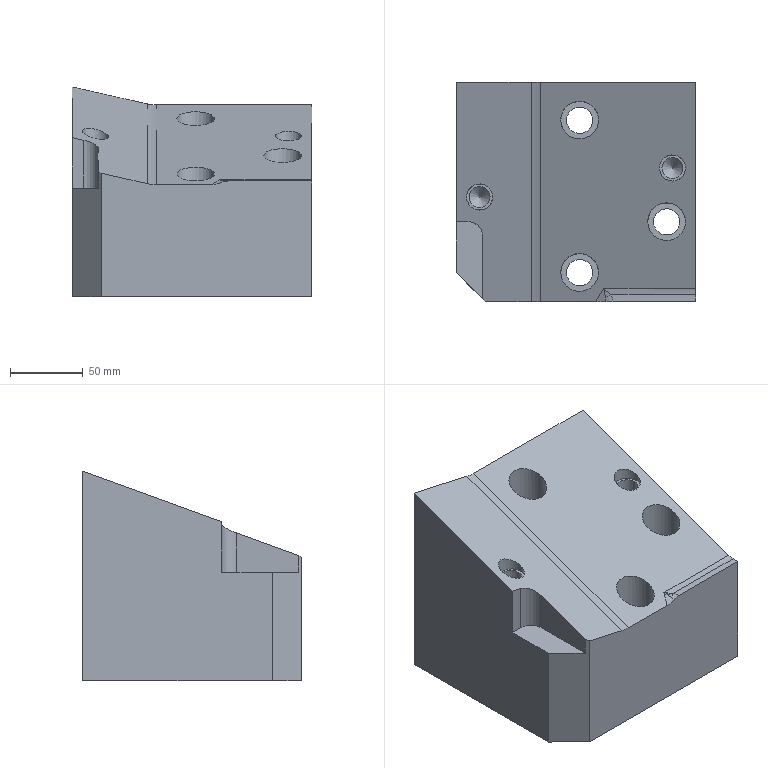Part | STEP file | lll_id5030_x_t | 1 solid | 53 faces | box 165 x 151 x 144.814 mm | volume 2436830 mm3 | plane 23 | cylinder 22 | torus 4 | cone 2 | spline 2 | commonest cylinder face diameters 25 x6 2 x4 18.009 x3 26.008 x3 14.506 x2 18 x2
STEP:
#1=CARTESIAN_POINT('',(2684.,105.,27.683));
#2=VERTEX_POINT('',#1);
#3=CARTESIAN_POINT('',(2684.,114.,30.959));
#4=DIRECTION('',(0.,-0.342,0.9397));
#5=DIRECTION('',(0.,-0.9397,-0.342));
#6=AXIS2_PLACEMENT_3D('',#3,#4,#5);
#7=ELLIPSE('',#6,9.578,9.);
#8=EDGE_CURVE('',#2,#2,#7,.T.);
#9=ORIENTED_EDGE('',*,*,#8,.F.);
#10=EDGE_LOOP('',(#9));
#11=FACE_BOUND('',#10,.T.);
#12=CARTESIAN_POINT('',(2620.,133.996,38.237));
#13=VERTEX_POINT('',#12);
#14=CARTESIAN_POINT('',(2620.,147.,42.97));
#15=DIRECTION('',(0.,-0.342,0.9397));
#16=DIRECTION('',(0.,-0.9397,-0.342));
#17=AXIS2_PLACEMENT_3D('',#14,#15,#16);
#18=ELLIPSE('',#17,13.839,13.004);
#19=EDGE_CURVE('',#13,#13,#18,.T.);
#20=ORIENTED_EDGE('',*,*,#19,.F.);
#21=EDGE_LOOP('',(#20));
#22=FACE_BOUND('',#21,.T.);
#23=CARTESIAN_POINT('',(2680.,63.996,12.759));
#24=VERTEX_POINT('',#23);
#25=CARTESIAN_POINT('',(2680.,77.,17.492));
#26=DIRECTION('',(0.,-0.342,0.9397));
#27=DIRECTION('',(0.,-0.9397,-0.342));
#28=AXIS2_PLACEMENT_3D('',#25,#26,#27);
#29=ELLIPSE('',#28,13.839,13.004);
#30=EDGE_CURVE('',#24,#24,#29,.T.);
#31=ORIENTED_EDGE('',*,*,#30,.F.);
#32=EDGE_LOOP('',(#31));
#33=FACE_BOUND('',#32,.T.);
#34=CARTESIAN_POINT('',(2620.,28.996,0.02));
#35=VERTEX_POINT('',#34);
#36=CARTESIAN_POINT('',(2620.,42.,4.753));
#37=DIRECTION('',(0.,-0.342,0.9397));
#38=DIRECTION('',(0.,-0.9397,-0.342));
#39=AXIS2_PLACEMENT_3D('',#36,#37,#38);
#40=ELLIPSE('',#39,13.839,13.004);
#41=EDGE_CURVE('',#35,#35,#40,.T.);
#42=ORIENTED_EDGE('',*,*,#41,.F.);
#43=EDGE_LOOP('',(#42));
#44=FACE_BOUND('',#43,.T.);
#45=CARTESIAN_POINT('',(2592.89,22.,-2.526));
#46=VERTEX_POINT('',#45);
#47=CARTESIAN_POINT('',(2630.969,22.,-2.526));
#48=VERTEX_POINT('',#47);
#49=CARTESIAN_POINT('',(2520.,22.,-2.526));
#50=DIRECTION('',(1.,0.,0.));
#51=VECTOR('',#50,1.);
#52=LINE('',#49,#51);
#53=EDGE_CURVE('',#46,#48,#52,.T.);
#54=ORIENTED_EDGE('',*,*,#53,.T.);
#55=CARTESIAN_POINT('',(2636.651,31.012,0.7538));
#56=VERTEX_POINT('',#55);
#57=CARTESIAN_POINT('',(2693.179,120.68,33.39));
#58=DIRECTION('',(0.5097,0.8085,0.2943));
#59=VECTOR('',#58,1.);
#60=LINE('',#57,#59);
#61=EDGE_CURVE('',#48,#56,#60,.T.);
#62=ORIENTED_EDGE('',*,*,#61,.T.);
#63=CARTESIAN_POINT('',(2700.,31.012,0.7538));
#64=VERTEX_POINT('',#63);
#65=CARTESIAN_POINT('',(2872.426,31.012,0.7538));
#66=DIRECTION('',(1.,0.,0.));
#67=VECTOR('',#66,1.);
#68=LINE('',#65,#67);
#69=EDGE_CURVE('',#56,#64,#68,.T.);
#70=ORIENTED_EDGE('',*,*,#69,.T.);
#71=CARTESIAN_POINT('',(2700.,173.,52.433));
#72=VERTEX_POINT('',#71);
#73=CARTESIAN_POINT('',(2700.,20.898,-2.927));
#74=DIRECTION('',(0.,0.9397,0.342));
#75=VECTOR('',#74,1.);
#76=LINE('',#73,#75);
#77=EDGE_CURVE('',#64,#72,#76,.T.);
#78=ORIENTED_EDGE('',*,*,#77,.T.);
#79=CARTESIAN_POINT('',(2592.89,173.,52.433));
#80=VERTEX_POINT('',#79);
#81=CARTESIAN_POINT('',(2872.426,173.,52.433));
#82=DIRECTION('',(-1.,0.,0.));
#83=VECTOR('',#82,1.);
#84=LINE('',#81,#83);
#85=EDGE_CURVE('',#72,#80,#84,.T.);
#86=ORIENTED_EDGE('',*,*,#85,.T.);
#87=CARTESIAN_POINT('',(2592.89,20.898,-2.927));
#88=DIRECTION('',(0.,-0.9397,-0.342));
#89=VECTOR('',#88,1.);
#90=LINE('',#87,#89);
#91=EDGE_CURVE('',#80,#46,#90,.T.);
#92=ORIENTED_EDGE('',*,*,#91,.T.);
#93=EDGE_LOOP('',(#54,#62,#70,#78,#86,#92));
#94=FACE_BOUND('',#93,.T.);
#95=CARTESIAN_POINT('',(2872.426,20.898,-2.927));
#96=DIRECTION('',(0.,-0.342,0.9397));
#97=DIRECTION('',(0.,0.9397,0.342));
#98=AXIS2_PLACEMENT_3D('',#95,#96,#97);
#99=PLANE('',#98);
#100=ADVANCED_FACE('',(#11,#22,#33,#44,#94),#99,.T.);
#101=CARTESIAN_POINT('',(2553.,24.,-5.));
#102=VERTEX_POINT('',#101);
#103=CARTESIAN_POINT('',(2553.,67.,-5.));
#104=VERTEX_POINT('',#103);
#105=CARTESIAN_POINT('',(2553.,67.,-5.));
#106=DIRECTION('',(0.,1.,0.));
#107=VECTOR('',#106,1.);
#108=LINE('',#105,#107);
#109=EDGE_CURVE('',#102,#104,#108,.T.);
#110=ORIENTED_EDGE('',*,*,#109,.F.);
#111=CARTESIAN_POINT('',(2553.,24.,6.511));
#112=VERTEX_POINT('',#111);
#113=CARTESIAN_POINT('',(2553.,24.,195.));
#114=DIRECTION('',(0.,0.,1.));
#115=VECTOR('',#114,1.);
#116=LINE('',#113,#115);
#117=EDGE_CURVE('',#102,#112,#116,.T.);
#118=ORIENTED_EDGE('',*,*,#117,.T.);
#119=CARTESIAN_POINT('',(2553.,67.,22.162));
#120=VERTEX_POINT('',#119);
#121=CARTESIAN_POINT('',(2553.,21.046,5.436));
#122=DIRECTION('',(0.,-0.9397,-0.342));
#123=VECTOR('',#122,1.);
#124=LINE('',#121,#123);
#125=EDGE_CURVE('',#120,#112,#124,.T.);
#126=ORIENTED_EDGE('',*,*,#125,.F.);
#127=CARTESIAN_POINT('',(2553.,67.,195.));
#128=DIRECTION('',(0.,0.,1.));
#129=VECTOR('',#128,1.);
#130=LINE('',#127,#129);
#131=EDGE_CURVE('',#104,#120,#130,.T.);
#132=ORIENTED_EDGE('',*,*,#131,.F.);
#133=EDGE_LOOP('',(#110,#118,#126,#132));
#134=FACE_OUTER_BOUND('',#133,.T.);
#135=CARTESIAN_POINT('',(2553.,67.,195.));
#136=DIRECTION('',(-1.,0.,0.));
#137=DIRECTION('',(0.,0.,-1.));
#138=AXIS2_PLACEMENT_3D('',#135,#136,#137);
#139=PLANE('',#138);
#140=ADVANCED_FACE('',(#134),#139,.T.);
#141=CARTESIAN_POINT('',(2543.,77.,-5.));
#142=VERTEX_POINT('',#141);
#143=CARTESIAN_POINT('',(2543.,77.,28.064));
#144=VERTEX_POINT('',#143);
#145=CARTESIAN_POINT('',(2543.,77.,195.));
#146=DIRECTION('',(0.,0.,1.));
#147=VECTOR('',#146,1.);
#148=LINE('',#145,#147);
#149=EDGE_CURVE('',#142,#144,#148,.T.);
#150=ORIENTED_EDGE('',*,*,#149,.F.);
#151=CARTESIAN_POINT('',(2543.,67.,-5.));
#152=DIRECTION('',(0.,0.,1.));
#153=DIRECTION('',(-1.,0.,0.));
#154=AXIS2_PLACEMENT_3D('',#151,#152,#153);
#155=CIRCLE('',#154,10.);
#156=EDGE_CURVE('',#104,#142,#155,.T.);
#157=ORIENTED_EDGE('',*,*,#156,.F.);
#158=ORIENTED_EDGE('',*,*,#131,.T.);
#159=CARTESIAN_POINT('',(2543.,67.,24.424));
#160=DIRECTION('',(-0.2079,0.3345,-0.9192));
#161=DIRECTION('',(0.4852,-0.7807,-0.3939));
#162=AXIS2_PLACEMENT_3D('',#159,#160,#161);
#163=ELLIPSE('',#162,10.88,10.);
#164=EDGE_CURVE('',#144,#120,#163,.T.);
#165=ORIENTED_EDGE('',*,*,#164,.F.);
#166=EDGE_LOOP('',(#150,#157,#158,#165));
#167=FACE_OUTER_BOUND('',#166,.T.);
#168=CARTESIAN_POINT('',(2543.,67.,195.));
#169=DIRECTION('',(0.,0.,-1.));
#170=DIRECTION('',(1.,0.,0.));
#171=AXIS2_PLACEMENT_3D('',#168,#169,#170);
#172=CYLINDRICAL_SURFACE('',#171,10.);
#173=ADVANCED_FACE('',(#167),#172,.F.);
#174=CARTESIAN_POINT('',(2535.,77.,29.873));
#175=VERTEX_POINT('',#174);
#176=CARTESIAN_POINT('',(2535.,77.,-5.));
#177=VERTEX_POINT('',#176);
#178=CARTESIAN_POINT('',(2535.,77.,195.));
#179=DIRECTION('',(0.,0.,-1.));
#180=VECTOR('',#179,1.);
#181=LINE('',#178,#180);
#182=EDGE_CURVE('',#175,#177,#181,.T.);
#183=ORIENTED_EDGE('',*,*,#182,.T.);
#184=CARTESIAN_POINT('',(2535.,77.,-5.));
#185=DIRECTION('',(-1.,0.,0.));
#186=VECTOR('',#185,1.);
#187=LINE('',#184,#186);
#188=EDGE_CURVE('',#142,#177,#187,.T.);
#189=ORIENTED_EDGE('',*,*,#188,.F.);
#190=ORIENTED_EDGE('',*,*,#149,.T.);
#191=CARTESIAN_POINT('',(2590.843,77.,17.242));
#192=DIRECTION('',(0.9754,0.,-0.2206));
#193=VECTOR('',#192,1.);
#194=LINE('',#191,#193);
#195=EDGE_CURVE('',#175,#144,#194,.T.);
#196=ORIENTED_EDGE('',*,*,#195,.F.);
#197=EDGE_LOOP('',(#183,#189,#190,#196));
#198=FACE_OUTER_BOUND('',#197,.T.);
#199=CARTESIAN_POINT('',(2535.,77.,195.));
#200=DIRECTION('',(0.,-1.,0.));
#201=DIRECTION('',(0.,0.,-1.));
#202=AXIS2_PLACEMENT_3D('',#199,#200,#201);
#203=PLANE('',#202);
#204=ADVANCED_FACE('',(#198),#203,.T.);
#205=CARTESIAN_POINT('',(2535.,42.,-5.));
#206=VERTEX_POINT('',#205);
#207=CARTESIAN_POINT('',(2535.,77.,-5.));
#208=DIRECTION('',(0.,-1.,0.));
#209=VECTOR('',#208,1.);
#210=LINE('',#207,#209);
#211=EDGE_CURVE('',#177,#206,#210,.T.);
#212=ORIENTED_EDGE('',*,*,#211,.T.);
#213=CARTESIAN_POINT('',(2526.5,50.5,-5.));
#214=DIRECTION('',(0.7071,-0.7071,0.));
#215=VECTOR('',#214,1.);
#216=LINE('',#213,#215);
#217=EDGE_CURVE('',#206,#102,#216,.T.);
#218=ORIENTED_EDGE('',*,*,#217,.T.);
#219=ORIENTED_EDGE('',*,*,#109,.T.);
#220=ORIENTED_EDGE('',*,*,#156,.T.);
#221=ORIENTED_EDGE('',*,*,#188,.T.);
#222=EDGE_LOOP('',(#212,#218,#219,#220,#221));
#223=FACE_OUTER_BOUND('',#222,.T.);
#224=CARTESIAN_POINT('',(2543.,67.,-5.));
#225=DIRECTION('',(0.,0.,1.));
#226=DIRECTION('',(-1.,0.,0.));
#227=AXIS2_PLACEMENT_3D('',#224,#225,#226);
#228=PLANE('',#227);
#229=ADVANCED_FACE('',(#223),#228,.T.);
#230=CARTESIAN_POINT('',(2555.751,86.356,28.585));
#231=VERTEX_POINT('',#230);
#232=CARTESIAN_POINT('',(2551.,94.,32.442));
#233=DIRECTION('',(0.2079,-0.3345,0.9192));
#234=DIRECTION('',(0.4852,-0.7807,-0.3939));
#235=AXIS2_PLACEMENT_3D('',#232,#233,#234);
#236=ELLIPSE('',#235,9.792,9.);
#237=EDGE_CURVE('',#231,#231,#236,.T.);
#238=ORIENTED_EDGE('',*,*,#237,.F.);
#239=EDGE_LOOP('',(#238));
#240=FACE_BOUND('',#239,.T.);
#241=ORIENTED_EDGE('',*,*,#125,.T.);
#242=CARTESIAN_POINT('',(2555.,22.,5.331));
#243=VERTEX_POINT('',#242);
#244=CARTESIAN_POINT('',(2569.506,7.494,-3.23));
#245=DIRECTION('',(0.6526,-0.6526,-0.3851));
#246=VECTOR('',#245,1.);
#247=LINE('',#244,#246);
#248=EDGE_CURVE('',#112,#243,#247,.T.);
#249=ORIENTED_EDGE('',*,*,#248,.T.);
#250=CARTESIAN_POINT('',(2586.652,22.,-1.829));
#251=VERTEX_POINT('',#250);
#252=CARTESIAN_POINT('',(2540.066,22.,8.709));
#253=DIRECTION('',(0.9754,0.,-0.2206));
#254=VECTOR('',#253,1.);
#255=LINE('',#252,#254);
#256=EDGE_CURVE('',#243,#251,#255,.T.);
#257=ORIENTED_EDGE('',*,*,#256,.T.);
#258=CARTESIAN_POINT('',(2586.652,173.,53.131));
#259=VERTEX_POINT('',#258);
#260=CARTESIAN_POINT('',(2586.652,205.677,65.024));
#261=DIRECTION('',(0.,-0.9397,-0.342));
#262=VECTOR('',#261,1.);
#263=LINE('',#260,#262);
#264=EDGE_CURVE('',#259,#251,#263,.T.);
#265=ORIENTED_EDGE('',*,*,#264,.F.);
#266=CARTESIAN_POINT('',(2535.,173.,64.814));
#267=VERTEX_POINT('',#266);
#268=CARTESIAN_POINT('',(2598.362,173.,50.482));
#269=DIRECTION('',(-0.9754,0.,0.2206));
#270=VECTOR('',#269,1.);
#271=LINE('',#268,#270);
#272=EDGE_CURVE('',#259,#267,#271,.T.);
#273=ORIENTED_EDGE('',*,*,#272,.T.);
#274=CARTESIAN_POINT('',(2535.,19.738,9.032));
#275=DIRECTION('',(0.,0.9397,0.342));
#276=VECTOR('',#275,1.);
#277=LINE('',#274,#276);
#278=EDGE_CURVE('',#175,#267,#277,.T.);
#279=ORIENTED_EDGE('',*,*,#278,.F.);
#280=ORIENTED_EDGE('',*,*,#195,.T.);
#281=ORIENTED_EDGE('',*,*,#164,.T.);
#282=EDGE_LOOP('',(#241,#249,#257,#265,#273,#279,#280,#281));
#283=FACE_BOUND('',#282,.T.);
#284=CARTESIAN_POINT('',(2586.652,23.493,-1.285));
#285=DIRECTION('',(0.2079,-0.3345,0.9192));
#286=DIRECTION('',(0.,0.9397,0.342));
#287=AXIS2_PLACEMENT_3D('',#284,#285,#286);
#288=PLANE('',#287);
#289=ADVANCED_FACE('',(#240,#283),#288,.T.);
#290=ORIENTED_EDGE('',*,*,#91,.F.);
#291=CARTESIAN_POINT('',(2592.89,173.,84.359));
#292=DIRECTION('',(0.,1.,0.));
#293=DIRECTION('',(0.,0.,-1.));
#294=AXIS2_PLACEMENT_3D('',#291,#292,#293);
#295=ELLIPSE('',#294,31.925,30.);
#296=EDGE_CURVE('',#80,#259,#295,.T.);
#297=ORIENTED_EDGE('',*,*,#296,.T.);
#298=ORIENTED_EDGE('',*,*,#264,.T.);
#299=CARTESIAN_POINT('',(2592.89,22.,29.399));
#300=DIRECTION('',(0.,1.,0.));
#301=DIRECTION('',(0.,0.,-1.));
#302=AXIS2_PLACEMENT_3D('',#299,#300,#301);
#303=ELLIPSE('',#302,31.925,30.);
#304=EDGE_CURVE('',#46,#251,#303,.T.);
#305=ORIENTED_EDGE('',*,*,#304,.F.);
#306=EDGE_LOOP('',(#290,#297,#298,#305));
#307=FACE_OUTER_BOUND('',#306,.T.);
#308=CARTESIAN_POINT('',(2592.89,195.641,92.599));
#309=DIRECTION('',(0.,-0.9397,-0.342));
#310=DIRECTION('',(0.,-0.342,0.9397));
#311=AXIS2_PLACEMENT_3D('',#308,#309,#310);
#312=CYLINDRICAL_SURFACE('',#311,30.);
#313=ADVANCED_FACE('',(#307),#312,.F.);
#314=CARTESIAN_POINT('',(2535.,173.,-80.));
#315=VERTEX_POINT('',#314);
#316=CARTESIAN_POINT('',(2535.,42.,-80.));
#317=VERTEX_POINT('',#316);
#318=CARTESIAN_POINT('',(2535.,-1.,-80.));
#319=DIRECTION('',(0.,-1.,0.));
#320=VECTOR('',#319,1.);
#321=LINE('',#318,#320);
#322=EDGE_CURVE('',#315,#317,#321,.T.);
#323=ORIENTED_EDGE('',*,*,#322,.T.);
#324=CARTESIAN_POINT('',(2535.,42.,-80.));
#325=DIRECTION('',(0.,0.,1.));
#326=VECTOR('',#325,1.);
#327=LINE('',#324,#326);
#328=EDGE_CURVE('',#317,#206,#327,.T.);
#329=ORIENTED_EDGE('',*,*,#328,.T.);
#330=ORIENTED_EDGE('',*,*,#211,.F.);
#331=ORIENTED_EDGE('',*,*,#182,.F.);
#332=ORIENTED_EDGE('',*,*,#278,.T.);
#333=CARTESIAN_POINT('',(2535.,173.,-80.));
#334=DIRECTION('',(0.,0.,-1.));
#335=VECTOR('',#334,1.);
#336=LINE('',#333,#335);
#337=EDGE_CURVE('',#267,#315,#336,.T.);
#338=ORIENTED_EDGE('',*,*,#337,.T.);
#339=EDGE_LOOP('',(#323,#329,#330,#331,#332,#338));
#340=FACE_OUTER_BOUND('',#339,.T.);
#341=CARTESIAN_POINT('',(2535.,335.,-80.));
#342=DIRECTION('',(1.,0.,0.));
#343=DIRECTION('',(0.,0.,1.));
#344=AXIS2_PLACEMENT_3D('',#341,#342,#343);
#345=PLANE('',#344);
#346=ADVANCED_FACE('',(#340),#345,.F.);
#347=CARTESIAN_POINT('',(2552.5,115.5,-80.));
#348=VERTEX_POINT('',#347);
#349=CARTESIAN_POINT('',(2577.5,115.5,-80.));
#350=VERTEX_POINT('',#349);
#351=CARTESIAN_POINT('',(2565.,115.5,-80.));
#352=DIRECTION('',(0.,0.,-1.));
#353=DIRECTION('',(-1.,0.,0.));
#354=AXIS2_PLACEMENT_3D('',#351,#352,#353);
#355=CIRCLE('',#354,12.5);
#356=EDGE_CURVE('',#348,#350,#355,.T.);
#357=ORIENTED_EDGE('',*,*,#356,.F.);
#358=CARTESIAN_POINT('',(2552.5,59.5,-80.));
#359=VERTEX_POINT('',#358);
#360=CARTESIAN_POINT('',(2552.5,-1.,-80.));
#361=DIRECTION('',(0.,1.,0.));
#362=VECTOR('',#361,1.);
#363=LINE('',#360,#362);
#364=EDGE_CURVE('',#359,#348,#363,.T.);
#365=ORIENTED_EDGE('',*,*,#364,.F.);
#366=CARTESIAN_POINT('',(2577.5,59.5,-80.));
#367=VERTEX_POINT('',#366);
#368=CARTESIAN_POINT('',(2565.,59.5,-80.));
#369=DIRECTION('',(0.,0.,-1.));
#370=DIRECTION('',(-1.,0.,0.));
#371=AXIS2_PLACEMENT_3D('',#368,#369,#370);
#372=CIRCLE('',#371,12.5);
#373=EDGE_CURVE('',#367,#359,#372,.T.);
#374=ORIENTED_EDGE('',*,*,#373,.F.);
#375=CARTESIAN_POINT('',(2577.5,-1.,-80.));
#376=DIRECTION('',(0.,-1.,0.));
#377=VECTOR('',#376,1.);
#378=LINE('',#375,#377);
#379=EDGE_CURVE('',#350,#367,#378,.T.);
#380=ORIENTED_EDGE('',*,*,#379,.F.);
#381=EDGE_LOOP('',(#357,#365,#374,#380));
#382=FACE_BOUND('',#381,.T.);
#383=CARTESIAN_POINT('',(2621.,100.5,-80.));
#384=VERTEX_POINT('',#383);
#385=CARTESIAN_POINT('',(2621.,125.5,-80.));
#386=VERTEX_POINT('',#385);
#387=CARTESIAN_POINT('',(2621.,113.,-80.));
#388=DIRECTION('',(0.,0.,-1.));
#389=DIRECTION('',(-1.,0.,0.));
#390=AXIS2_PLACEMENT_3D('',#387,#388,#389);
#391=CIRCLE('',#390,12.5);
#392=EDGE_CURVE('',#384,#386,#391,.T.);
#393=ORIENTED_EDGE('',*,*,#392,.F.);
#394=CARTESIAN_POINT('',(2677.,100.5,-80.));
#395=VERTEX_POINT('',#394);
#396=CARTESIAN_POINT('',(-2196.249,100.5,-80.));
#397=DIRECTION('',(-1.,0.,0.));
#398=VECTOR('',#397,1.);
#399=LINE('',#396,#398);
#400=EDGE_CURVE('',#395,#384,#399,.T.);
#401=ORIENTED_EDGE('',*,*,#400,.F.);
#402=CARTESIAN_POINT('',(2677.,125.5,-80.));
#403=VERTEX_POINT('',#402);
#404=CARTESIAN_POINT('',(2677.,113.,-80.));
#405=DIRECTION('',(0.,0.,-1.));
#406=DIRECTION('',(-1.,0.,0.));
#407=AXIS2_PLACEMENT_3D('',#404,#405,#406);
#408=CIRCLE('',#407,12.5);
#409=EDGE_CURVE('',#403,#395,#408,.T.);
#410=ORIENTED_EDGE('',*,*,#409,.F.);
#411=CARTESIAN_POINT('',(-2196.249,125.5,-80.));
#412=DIRECTION('',(1.,0.,0.));
#413=VECTOR('',#412,1.);
#414=LINE('',#411,#413);
#415=EDGE_CURVE('',#386,#403,#414,.T.);
#416=ORIENTED_EDGE('',*,*,#415,.F.);
#417=EDGE_LOOP('',(#393,#401,#410,#416));
#418=FACE_BOUND('',#417,.T.);
#419=CARTESIAN_POINT('',(2555.,22.,-80.));
#420=VERTEX_POINT('',#419);
#421=CARTESIAN_POINT('',(2700.,22.,-80.));
#422=VERTEX_POINT('',#421);
#423=CARTESIAN_POINT('',(-2196.249,22.,-80.));
#424=DIRECTION('',(1.,0.,0.));
#425=VECTOR('',#424,1.);
#426=LINE('',#423,#425);
#427=EDGE_CURVE('',#420,#422,#426,.T.);
#428=ORIENTED_EDGE('',*,*,#427,.F.);
#429=CARTESIAN_POINT('',(190.875,2386.125,-80.));
#430=DIRECTION('',(-0.7071,0.7071,0.));
#431=VECTOR('',#430,1.);
#432=LINE('',#429,#431);
#433=EDGE_CURVE('',#420,#317,#432,.T.);
#434=ORIENTED_EDGE('',*,*,#433,.T.);
#435=ORIENTED_EDGE('',*,*,#322,.F.);
#436=CARTESIAN_POINT('',(2700.,173.,-80.));
#437=VERTEX_POINT('',#436);
#438=CARTESIAN_POINT('',(-2196.249,173.,-80.));
#439=DIRECTION('',(1.,0.,0.));
#440=VECTOR('',#439,1.);
#441=LINE('',#438,#440);
#442=EDGE_CURVE('',#315,#437,#441,.T.);
#443=ORIENTED_EDGE('',*,*,#442,.T.);
#444=CARTESIAN_POINT('',(2700.,-1.,-80.));
#445=DIRECTION('',(0.,1.,0.));
#446=VECTOR('',#445,1.);
#447=LINE('',#444,#446);
#448=EDGE_CURVE('',#422,#437,#447,.T.);
#449=ORIENTED_EDGE('',*,*,#448,.F.);
#450=EDGE_LOOP('',(#428,#434,#435,#443,#449));
#451=FACE_BOUND('',#450,.T.);
#452=CARTESIAN_POINT('',(2629.005,42.,-80.));
#453=VERTEX_POINT('',#452);
#454=CARTESIAN_POINT('',(2620.,42.,-80.));
#455=DIRECTION('',(0.,0.,-1.));
#456=DIRECTION('',(1.,0.,0.));
#457=AXIS2_PLACEMENT_3D('',#454,#455,#456);
#458=CIRCLE('',#457,9.005);
#459=EDGE_CURVE('',#453,#453,#458,.T.);
#460=ORIENTED_EDGE('',*,*,#459,.F.);
#461=EDGE_LOOP('',(#460));
#462=FACE_BOUND('',#461,.T.);
#463=CARTESIAN_POINT('',(2689.005,77.,-80.));
#464=VERTEX_POINT('',#463);
#465=CARTESIAN_POINT('',(2680.,77.,-80.));
#466=DIRECTION('',(0.,0.,-1.));
#467=DIRECTION('',(1.,0.,0.));
#468=AXIS2_PLACEMENT_3D('',#465,#466,#467);
#469=CIRCLE('',#468,9.005);
#470=EDGE_CURVE('',#464,#464,#469,.T.);
#471=ORIENTED_EDGE('',*,*,#470,.F.);
#472=EDGE_LOOP('',(#471));
#473=FACE_BOUND('',#472,.T.);
#474=CARTESIAN_POINT('',(2629.005,147.,-80.));
#475=VERTEX_POINT('',#474);
#476=CARTESIAN_POINT('',(2620.,147.,-80.));
#477=DIRECTION('',(0.,0.,-1.));
#478=DIRECTION('',(1.,0.,0.));
#479=AXIS2_PLACEMENT_3D('',#476,#477,#478);
#480=CIRCLE('',#479,9.005);
#481=EDGE_CURVE('',#475,#475,#480,.T.);
#482=ORIENTED_EDGE('',*,*,#481,.F.);
#483=EDGE_LOOP('',(#482));
#484=FACE_BOUND('',#483,.T.);
#485=CARTESIAN_POINT('',(-2196.249,-1.,-80.));
#486=DIRECTION('',(0.,0.,-1.));
#487=DIRECTION('',(1.,0.,0.));
#488=AXIS2_PLACEMENT_3D('',#485,#486,#487);
#489=PLANE('',#488);
#490=ADVANCED_FACE('',(#382,#418,#451,#462,#473,#484),#489,.T.);
#491=ORIENTED_EDGE('',*,*,#256,.F.);
#492=CARTESIAN_POINT('',(2555.,22.,-80.));
#493=DIRECTION('',(0.,0.,-1.));
#494=VECTOR('',#493,1.);
#495=LINE('',#492,#494);
#496=EDGE_CURVE('',#243,#420,#495,.T.);
#497=ORIENTED_EDGE('',*,*,#496,.T.);
#498=ORIENTED_EDGE('',*,*,#427,.T.);
#499=CARTESIAN_POINT('',(2700.,22.,0.));
#500=VERTEX_POINT('',#499);
#501=CARTESIAN_POINT('',(2700.,22.,-80.));
#502=DIRECTION('',(0.,0.,-1.));
#503=VECTOR('',#502,1.);
#504=LINE('',#501,#503);
#505=EDGE_CURVE('',#500,#422,#504,.T.);
#506=ORIENTED_EDGE('',*,*,#505,.F.);
#507=CARTESIAN_POINT('',(2643.022,22.,0.));
#508=VERTEX_POINT('',#507);
#509=CARTESIAN_POINT('',(13174.883,22.,0.));
#510=DIRECTION('',(1.,0.,0.));
#511=VECTOR('',#510,1.);
#512=LINE('',#509,#511);
#513=EDGE_CURVE('',#508,#500,#512,.T.);
#514=ORIENTED_EDGE('',*,*,#513,.F.);
#515=CARTESIAN_POINT('',(2637.906,22.,-1.056));
#516=VERTEX_POINT('',#515);
#517=CARTESIAN_POINT('',(2643.022,22.,0.));
#518=CARTESIAN_POINT('',(2642.559,22.,-0.000000003));
#519=CARTESIAN_POINT('',(2642.096,22.,-0.02511));
#520=CARTESIAN_POINT('',(2641.636,22.,-0.07498));
#521=CARTESIAN_POINT('',(2641.176,22.,-0.1249));
#522=CARTESIAN_POINT('',(2640.718,22.,-0.1996));
#523=CARTESIAN_POINT('',(2640.266,22.,-0.2985));
#524=CARTESIAN_POINT('',(2639.459,22.,-0.4751));
#525=CARTESIAN_POINT('',(2638.665,22.,-0.7303));
#526=CARTESIAN_POINT('',(2637.906,22.,-1.056));
#527=B_SPLINE_CURVE_WITH_KNOTS('',3,(#517,#518,#519,#520,#521,#522,#523,#524,#525,#526),.UNSPECIFIED.,.F.,.F.,(4,3,3,4),(0.,0.2638,0.5276,1.),.UNSPECIFIED.);
#528=EDGE_CURVE('',#508,#516,#527,.T.);
#529=ORIENTED_EDGE('',*,*,#528,.T.);
#530=CARTESIAN_POINT('',(2633.664,22.,10.776));
#531=DIRECTION('',(0.,1.,0.));
#532=DIRECTION('',(0.866,0.,0.5));
#533=AXIS2_PLACEMENT_3D('',#530,#531,#532);
#534=ELLIPSE('',#533,15.461,12.5);
#535=EDGE_CURVE('',#516,#48,#534,.T.);
#536=ORIENTED_EDGE('',*,*,#535,.T.);
#537=ORIENTED_EDGE('',*,*,#53,.F.);
#538=ORIENTED_EDGE('',*,*,#304,.T.);
#539=EDGE_LOOP('',(#491,#497,#498,#506,#514,#529,#536,#537,#538));
#540=FACE_OUTER_BOUND('',#539,.T.);
#541=CARTESIAN_POINT('',(2520.,22.,-80.));
#542=DIRECTION('',(0.,1.,0.));
#543=DIRECTION('',(0.,0.,1.));
#544=AXIS2_PLACEMENT_3D('',#541,#542,#543);
#545=PLANE('',#544);
#546=ADVANCED_FACE('',(#540),#545,.F.);
#547=CARTESIAN_POINT('',(2700.,173.,6.));
#548=DIRECTION('',(0.,0.,1.));
#549=VECTOR('',#548,1.);
#550=LINE('',#547,#549);
#551=EDGE_CURVE('',#437,#72,#550,.T.);
#552=ORIENTED_EDGE('',*,*,#551,.F.);
#553=ORIENTED_EDGE('',*,*,#442,.F.);
#554=ORIENTED_EDGE('',*,*,#337,.F.);
#555=ORIENTED_EDGE('',*,*,#272,.F.);
#556=ORIENTED_EDGE('',*,*,#296,.F.);
#557=ORIENTED_EDGE('',*,*,#85,.F.);
#558=EDGE_LOOP('',(#552,#553,#554,#555,#556,#557));
#559=FACE_OUTER_BOUND('',#558,.T.);
#560=CARTESIAN_POINT('',(2692.5,173.,6.));
#561=DIRECTION('',(0.,1.,0.));
#562=DIRECTION('',(0.,0.,-1.));
#563=AXIS2_PLACEMENT_3D('',#560,#561,#562);
#564=PLANE('',#563);
#565=ADVANCED_FACE('',(#559),#564,.T.);
#566=ORIENTED_EDGE('',*,*,#448,.T.);
#567=ORIENTED_EDGE('',*,*,#551,.T.);
#568=ORIENTED_EDGE('',*,*,#77,.F.);
#569=CARTESIAN_POINT('',(2700.,26.737,0.));
#570=VERTEX_POINT('',#569);
#571=CARTESIAN_POINT('',(2700.,26.737,12.5));
#572=DIRECTION('',(-1.,0.,0.));
#573=DIRECTION('',(0.,0.,-1.));
#574=AXIS2_PLACEMENT_3D('',#571,#572,#573);
#575=CIRCLE('',#574,12.5);
#576=EDGE_CURVE('',#64,#570,#575,.T.);
#577=ORIENTED_EDGE('',*,*,#576,.T.);
#578=CARTESIAN_POINT('',(2700.,20.,0.));
#579=DIRECTION('',(0.,1.,0.));
#580=VECTOR('',#579,1.);
#581=LINE('',#578,#580);
#582=EDGE_CURVE('',#500,#570,#581,.T.);
#583=ORIENTED_EDGE('',*,*,#582,.F.);
#584=ORIENTED_EDGE('',*,*,#505,.T.);
#585=EDGE_LOOP('',(#566,#567,#568,#577,#583,#584));
#586=FACE_OUTER_BOUND('',#585,.T.);
#587=CARTESIAN_POINT('',(2700.,97.5,-7.593));
#588=DIRECTION('',(-1.,0.,0.));
#589=DIRECTION('',(0.,0.,-1.));
#590=AXIS2_PLACEMENT_3D('',#587,#588,#589);
#591=PLANE('',#590);
#592=ADVANCED_FACE('',(#586),#591,.F.);
#593=CARTESIAN_POINT('',(2558.253,94.,25.814));
#594=VERTEX_POINT('',#593);
#595=CARTESIAN_POINT('',(2551.,94.,25.814));
#596=DIRECTION('',(0.,0.,-1.));
#597=DIRECTION('',(1.,0.,0.));
#598=AXIS2_PLACEMENT_3D('',#595,#596,#597);
#599=CIRCLE('',#598,7.253);
#600=EDGE_CURVE('',#594,#594,#599,.T.);
#601=ORIENTED_EDGE('',*,*,#600,.T.);
#602=EDGE_LOOP('',(#601));
#603=FACE_BOUND('',#602,.T.);
#604=CARTESIAN_POINT('',(2560.,94.,25.814));
#605=VERTEX_POINT('',#604);
#606=CARTESIAN_POINT('',(2551.,94.,25.814));
#607=DIRECTION('',(0.,0.,-1.));
#608=DIRECTION('',(1.,0.,0.));
#609=AXIS2_PLACEMENT_3D('',#606,#607,#608);
#610=CIRCLE('',#609,9.);
#611=EDGE_CURVE('',#605,#605,#610,.T.);
#612=ORIENTED_EDGE('',*,*,#611,.F.);
#613=EDGE_LOOP('',(#612));
#614=FACE_BOUND('',#613,.T.);
#615=CARTESIAN_POINT('',(2551.,94.,25.814));
#616=DIRECTION('',(0.,0.,-1.));
#617=DIRECTION('',(1.,0.,0.));
#618=AXIS2_PLACEMENT_3D('',#615,#616,#617);
#619=PLANE('',#618);
#620=ADVANCED_FACE('',(#603,#614),#619,.F.);
#621=ORIENTED_EDGE('',*,*,#237,.T.);
#622=EDGE_LOOP('',(#621));
#623=FACE_BOUND('',#622,.T.);
#624=ORIENTED_EDGE('',*,*,#611,.T.);
#625=EDGE_LOOP('',(#624));
#626=FACE_BOUND('',#625,.T.);
#627=CARTESIAN_POINT('',(2551.,94.,35.814));
#628=DIRECTION('',(0.,0.,-1.));
#629=DIRECTION('',(-1.,0.,0.));
#630=AXIS2_PLACEMENT_3D('',#627,#628,#629);
#631=CYLINDRICAL_SURFACE('',#630,9.);
#632=ADVANCED_FACE('',(#623,#626),#631,.F.);
#633=CARTESIAN_POINT('',(2691.253,114.,25.814));
#634=VERTEX_POINT('',#633);
#635=CARTESIAN_POINT('',(2684.,114.,25.814));
#636=DIRECTION('',(0.,0.,-1.));
#637=DIRECTION('',(1.,0.,0.));
#638=AXIS2_PLACEMENT_3D('',#635,#636,#637);
#639=CIRCLE('',#638,7.253);
#640=EDGE_CURVE('',#634,#634,#639,.T.);
#641=ORIENTED_EDGE('',*,*,#640,.T.);
#642=EDGE_LOOP('',(#641));
#643=FACE_BOUND('',#642,.T.);
#644=CARTESIAN_POINT('',(2693.,114.,25.814));
#645=VERTEX_POINT('',#644);
#646=CARTESIAN_POINT('',(2684.,114.,25.814));
#647=DIRECTION('',(0.,0.,-1.));
#648=DIRECTION('',(1.,0.,0.));
#649=AXIS2_PLACEMENT_3D('',#646,#647,#648);
#650=CIRCLE('',#649,9.);
#651=EDGE_CURVE('',#645,#645,#650,.T.);
#652=ORIENTED_EDGE('',*,*,#651,.F.);
#653=EDGE_LOOP('',(#652));
#654=FACE_BOUND('',#653,.T.);
#655=CARTESIAN_POINT('',(2684.,114.,25.814));
#656=DIRECTION('',(0.,0.,-1.));
#657=DIRECTION('',(1.,0.,0.));
#658=AXIS2_PLACEMENT_3D('',#655,#656,#657);
#659=PLANE('',#658);
#660=ADVANCED_FACE('',(#643,#654),#659,.F.);
#661=ORIENTED_EDGE('',*,*,#8,.T.);
#662=EDGE_LOOP('',(#661));
#663=FACE_BOUND('',#662,.T.);
#664=ORIENTED_EDGE('',*,*,#651,.T.);
#665=EDGE_LOOP('',(#664));
#666=FACE_BOUND('',#665,.T.);
#667=CARTESIAN_POINT('',(2684.,114.,35.814));
#668=DIRECTION('',(0.,0.,-1.));
#669=DIRECTION('',(-1.,0.,0.));
#670=AXIS2_PLACEMENT_3D('',#667,#668,#669);
#671=CYLINDRICAL_SURFACE('',#670,9.);
#672=ADVANCED_FACE('',(#663,#666),#671,.F.);
#673=CARTESIAN_POINT('',(2676.747,114.,-1.939));
#674=VERTEX_POINT('',#673);
#675=CARTESIAN_POINT('',(2684.,114.,-1.939));
#676=DIRECTION('',(0.,0.,1.));
#677=DIRECTION('',(-1.,0.,0.));
#678=AXIS2_PLACEMENT_3D('',#675,#676,#677);
#679=CIRCLE('',#678,7.253);
#680=EDGE_CURVE('',#674,#674,#679,.T.);
#681=ORIENTED_EDGE('',*,*,#680,.F.);
#682=EDGE_LOOP('',(#681));
#683=FACE_BOUND('',#682,.T.);
#684=ORIENTED_EDGE('',*,*,#640,.F.);
#685=EDGE_LOOP('',(#684));
#686=FACE_BOUND('',#685,.T.);
#687=CARTESIAN_POINT('',(2684.,114.,35.814));
#688=DIRECTION('',(0.,0.,-1.));
#689=DIRECTION('',(1.,0.,0.));
#690=AXIS2_PLACEMENT_3D('',#687,#688,#689);
#691=CYLINDRICAL_SURFACE('',#690,7.253);
#692=ADVANCED_FACE('',(#683,#686),#691,.F.);
#693=CARTESIAN_POINT('',(2684.,114.,-9.192));
#694=VERTEX_POINT('',#693);
#695=VERTEX_LOOP('',#694);
#696=FACE_BOUND('',#695,.T.);
#697=ORIENTED_EDGE('',*,*,#680,.T.);
#698=EDGE_LOOP('',(#697));
#699=FACE_BOUND('',#698,.T.);
#700=CARTESIAN_POINT('',(2684.,114.,-1.939));
#701=DIRECTION('',(0.,0.,1.));
#702=DIRECTION('',(1.,0.,0.));
#703=AXIS2_PLACEMENT_3D('',#700,#701,#702);
#704=CONICAL_SURFACE('',#703,7.253,45.);
#705=ADVANCED_FACE('',(#696,#699),#704,.F.);
#706=CARTESIAN_POINT('',(2558.253,94.,-1.939));
#707=VERTEX_POINT('',#706);
#708=CARTESIAN_POINT('',(2551.,94.,-1.939));
#709=DIRECTION('',(0.,0.,-1.));
#710=DIRECTION('',(1.,0.,0.));
#711=AXIS2_PLACEMENT_3D('',#708,#709,#710);
#712=CIRCLE('',#711,7.253);
#713=EDGE_CURVE('',#707,#707,#712,.T.);
#714=ORIENTED_EDGE('',*,*,#713,.T.);
#715=EDGE_LOOP('',(#714));
#716=FACE_BOUND('',#715,.T.);
#717=ORIENTED_EDGE('',*,*,#600,.F.);
#718=EDGE_LOOP('',(#717));
#719=FACE_BOUND('',#718,.T.);
#720=CARTESIAN_POINT('',(2551.,94.,35.814));
#721=DIRECTION('',(0.,0.,-1.));
#722=DIRECTION('',(-1.,0.,0.));
#723=AXIS2_PLACEMENT_3D('',#720,#721,#722);
#724=CYLINDRICAL_SURFACE('',#723,7.253);
#725=ADVANCED_FACE('',(#716,#719),#724,.F.);
#726=CARTESIAN_POINT('',(2551.,94.,-9.192));
#727=VERTEX_POINT('',#726);
#728=VERTEX_LOOP('',#727);
#729=FACE_BOUND('',#728,.T.);
#730=ORIENTED_EDGE('',*,*,#713,.F.);
#731=EDGE_LOOP('',(#730));
#732=FACE_BOUND('',#731,.T.);
#733=CARTESIAN_POINT('',(2551.,94.,-1.939));
#734=DIRECTION('',(0.,0.,1.));
#735=DIRECTION('',(-1.,0.,0.));
#736=AXIS2_PLACEMENT_3D('',#733,#734,#735);
#737=CONICAL_SURFACE('',#736,7.253,45.);
#738=ADVANCED_FACE('',(#729,#732),#737,.F.);
#739=ORIENTED_EDGE('',*,*,#481,.T.);
#740=EDGE_LOOP('',(#739));
#741=FACE_BOUND('',#740,.T.);
#742=CARTESIAN_POINT('',(2629.005,147.,-40.));
#743=VERTEX_POINT('',#742);
#744=CARTESIAN_POINT('',(2620.,147.,-40.));
#745=DIRECTION('',(0.,0.,-1.));
#746=DIRECTION('',(1.,0.,0.));
#747=AXIS2_PLACEMENT_3D('',#744,#745,#746);
#748=CIRCLE('',#747,9.005);
#749=EDGE_CURVE('',#743,#743,#748,.T.);
#750=ORIENTED_EDGE('',*,*,#749,.F.);
#751=EDGE_LOOP('',(#750));
#752=FACE_BOUND('',#751,.T.);
#753=CARTESIAN_POINT('',(2620.,147.,66.814));
#754=DIRECTION('',(0.,0.,-1.));
#755=DIRECTION('',(-1.,0.,0.));
#756=AXIS2_PLACEMENT_3D('',#753,#754,#755);
#757=CYLINDRICAL_SURFACE('',#756,9.005);
#758=ADVANCED_FACE('',(#741,#752),#757,.F.);
#759=ORIENTED_EDGE('',*,*,#749,.T.);
#760=EDGE_LOOP('',(#759));
#761=FACE_BOUND('',#760,.T.);
#762=CARTESIAN_POINT('',(2606.996,147.,-40.));
#763=VERTEX_POINT('',#762);
#764=CARTESIAN_POINT('',(2620.,147.,-40.));
#765=DIRECTION('',(0.,0.,-1.));
#766=DIRECTION('',(-1.,0.,0.));
#767=AXIS2_PLACEMENT_3D('',#764,#765,#766);
#768=CIRCLE('',#767,13.004);
#769=EDGE_CURVE('',#763,#763,#768,.T.);
#770=ORIENTED_EDGE('',*,*,#769,.F.);
#771=EDGE_LOOP('',(#770));
#772=FACE_BOUND('',#771,.T.);
#773=CARTESIAN_POINT('',(2620.,147.,-40.));
#774=DIRECTION('',(0.,0.,-1.));
#775=DIRECTION('',(1.,0.,0.));
#776=AXIS2_PLACEMENT_3D('',#773,#774,#775);
#777=PLANE('',#776);
#778=ADVANCED_FACE('',(#761,#772),#777,.F.);
#779=ORIENTED_EDGE('',*,*,#19,.T.);
#780=EDGE_LOOP('',(#779));
#781=FACE_BOUND('',#780,.T.);
#782=ORIENTED_EDGE('',*,*,#769,.T.);
#783=EDGE_LOOP('',(#782));
#784=FACE_BOUND('',#783,.T.);
#785=CARTESIAN_POINT('',(2620.,147.,64.814));
#786=DIRECTION('',(0.,0.,-1.));
#787=DIRECTION('',(-1.,0.,0.));
#788=AXIS2_PLACEMENT_3D('',#785,#786,#787);
#789=CYLINDRICAL_SURFACE('',#788,13.004);
#790=ADVANCED_FACE('',(#781,#784),#789,.F.);
#791=ORIENTED_EDGE('',*,*,#470,.T.);
#792=EDGE_LOOP('',(#791));
#793=FACE_BOUND('',#792,.T.);
#794=CARTESIAN_POINT('',(2689.005,77.,-40.));
#795=VERTEX_POINT('',#794);
#796=CARTESIAN_POINT('',(2680.,77.,-40.));
#797=DIRECTION('',(0.,0.,-1.));
#798=DIRECTION('',(1.,0.,0.));
#799=AXIS2_PLACEMENT_3D('',#796,#797,#798);
#800=CIRCLE('',#799,9.005);
#801=EDGE_CURVE('',#795,#795,#800,.T.);
#802=ORIENTED_EDGE('',*,*,#801,.F.);
#803=EDGE_LOOP('',(#802));
#804=FACE_BOUND('',#803,.T.);
#805=CARTESIAN_POINT('',(2680.,77.,66.814));
#806=DIRECTION('',(0.,0.,-1.));
#807=DIRECTION('',(-1.,0.,0.));
#808=AXIS2_PLACEMENT_3D('',#805,#806,#807);
#809=CYLINDRICAL_SURFACE('',#808,9.005);
#810=ADVANCED_FACE('',(#793,#804),#809,.F.);
#811=ORIENTED_EDGE('',*,*,#801,.T.);
#812=EDGE_LOOP('',(#811));
#813=FACE_BOUND('',#812,.T.);
#814=CARTESIAN_POINT('',(2666.996,77.,-40.));
#815=VERTEX_POINT('',#814);
#816=CARTESIAN_POINT('',(2680.,77.,-40.));
#817=DIRECTION('',(0.,0.,-1.));
#818=DIRECTION('',(-1.,0.,0.));
#819=AXIS2_PLACEMENT_3D('',#816,#817,#818);
#820=CIRCLE('',#819,13.004);
#821=EDGE_CURVE('',#815,#815,#820,.T.);
#822=ORIENTED_EDGE('',*,*,#821,.F.);
#823=EDGE_LOOP('',(#822));
#824=FACE_BOUND('',#823,.T.);
#825=CARTESIAN_POINT('',(2680.,77.,-40.));
#826=DIRECTION('',(0.,0.,-1.));
#827=DIRECTION('',(1.,0.,0.));
#828=AXIS2_PLACEMENT_3D('',#825,#826,#827);
#829=PLANE('',#828);
#830=ADVANCED_FACE('',(#813,#824),#829,.F.);
#831=ORIENTED_EDGE('',*,*,#30,.T.);
#832=EDGE_LOOP('',(#831));
#833=FACE_BOUND('',#832,.T.);
#834=ORIENTED_EDGE('',*,*,#821,.T.);
#835=EDGE_LOOP('',(#834));
#836=FACE_BOUND('',#835,.T.);
#837=CARTESIAN_POINT('',(2680.,77.,64.814));
#838=DIRECTION('',(0.,0.,-1.));
#839=DIRECTION('',(-1.,0.,0.));
#840=AXIS2_PLACEMENT_3D('',#837,#838,#839);
#841=CYLINDRICAL_SURFACE('',#840,13.004);
#842=ADVANCED_FACE('',(#833,#836),#841,.F.);
#843=ORIENTED_EDGE('',*,*,#459,.T.);
#844=EDGE_LOOP('',(#843));
#845=FACE_BOUND('',#844,.T.);
#846=CARTESIAN_POINT('',(2629.005,42.,-40.));
#847=VERTEX_POINT('',#846);
#848=CARTESIAN_POINT('',(2620.,42.,-40.));
#849=DIRECTION('',(0.,0.,-1.));
#850=DIRECTION('',(1.,0.,0.));
#851=AXIS2_PLACEMENT_3D('',#848,#849,#850);
#852=CIRCLE('',#851,9.005);
#853=EDGE_CURVE('',#847,#847,#852,.T.);
#854=ORIENTED_EDGE('',*,*,#853,.F.);
#855=EDGE_LOOP('',(#854));
#856=FACE_BOUND('',#855,.T.);
#857=CARTESIAN_POINT('',(2620.,42.,66.814));
#858=DIRECTION('',(0.,0.,-1.));
#859=DIRECTION('',(-1.,0.,0.));
#860=AXIS2_PLACEMENT_3D('',#857,#858,#859);
#861=CYLINDRICAL_SURFACE('',#860,9.005);
#862=ADVANCED_FACE('',(#845,#856),#861,.F.);
#863=ORIENTED_EDGE('',*,*,#853,.T.);
#864=EDGE_LOOP('',(#863));
#865=FACE_BOUND('',#864,.T.);
#866=CARTESIAN_POINT('',(2606.996,42.,-40.));
#867=VERTEX_POINT('',#866);
#868=CARTESIAN_POINT('',(2620.,42.,-40.));
#869=DIRECTION('',(0.,0.,-1.));
#870=DIRECTION('',(-1.,0.,0.));
#871=AXIS2_PLACEMENT_3D('',#868,#869,#870);
#872=CIRCLE('',#871,13.004);
#873=EDGE_CURVE('',#867,#867,#872,.T.);
#874=ORIENTED_EDGE('',*,*,#873,.F.);
#875=EDGE_LOOP('',(#874));
#876=FACE_BOUND('',#875,.T.);
#877=CARTESIAN_POINT('',(2620.,42.,-40.));
#878=DIRECTION('',(0.,0.,-1.));
#879=DIRECTION('',(1.,0.,0.));
#880=AXIS2_PLACEMENT_3D('',#877,#878,#879);
#881=PLANE('',#880);
#882=ADVANCED_FACE('',(#865,#876),#881,.F.);
#883=ORIENTED_EDGE('',*,*,#41,.T.);
#884=EDGE_LOOP('',(#883));
#885=FACE_BOUND('',#884,.T.);
#886=ORIENTED_EDGE('',*,*,#873,.T.);
#887=EDGE_LOOP('',(#886));
#888=FACE_BOUND('',#887,.T.);
#889=CARTESIAN_POINT('',(2620.,42.,64.814));
#890=DIRECTION('',(0.,0.,-1.));
#891=DIRECTION('',(-1.,0.,0.));
#892=AXIS2_PLACEMENT_3D('',#889,#890,#891);
#893=CYLINDRICAL_SURFACE('',#892,13.004);
#894=ADVANCED_FACE('',(#885,#888),#893,.F.);
#895=CARTESIAN_POINT('',(2641.524,26.737,0.));
#896=VERTEX_POINT('',#895);
#897=CARTESIAN_POINT('',(13174.883,26.737,0.));
#898=DIRECTION('',(-1.,0.,0.));
#899=VECTOR('',#898,1.);
#900=LINE('',#897,#899);
#901=EDGE_CURVE('',#570,#896,#900,.T.);
#902=ORIENTED_EDGE('',*,*,#901,.T.);
#903=CARTESIAN_POINT('',(2593.349,-41.95,0.));
#904=DIRECTION('',(0.,0.,-1.));
#905=DIRECTION('',(0.5333,0.8459,0.));
#906=AXIS2_PLACEMENT_3D('',#903,#904,#905);
#907=ELLIPSE('',#906,84.958,25.);
#908=EDGE_CURVE('',#896,#508,#907,.T.);
#909=ORIENTED_EDGE('',*,*,#908,.T.);
#910=ORIENTED_EDGE('',*,*,#513,.T.);
#911=ORIENTED_EDGE('',*,*,#582,.T.);
#912=EDGE_LOOP('',(#902,#909,#910,#911));
#913=FACE_OUTER_BOUND('',#912,.T.);
#914=CARTESIAN_POINT('',(13174.883,13720.786,0.));
#915=DIRECTION('',(0.,0.,-1.));
#916=DIRECTION('',(-1.,0.,0.));
#917=AXIS2_PLACEMENT_3D('',#914,#915,#916);
#918=PLANE('',#917);
#919=ADVANCED_FACE('',(#913),#918,.F.);
#920=ORIENTED_EDGE('',*,*,#69,.F.);
#921=CARTESIAN_POINT('',(2636.651,31.012,0.7538));
#922=CARTESIAN_POINT('',(2637.203,30.557,0.5881));
#923=CARTESIAN_POINT('',(2637.685,30.149,0.4692));
#924=CARTESIAN_POINT('',(2638.304,29.62,0.3357));
#925=CARTESIAN_POINT('',(2638.492,29.458,0.2988));
#926=CARTESIAN_POINT('',(2638.749,29.235,0.252));
#927=CARTESIAN_POINT('',(2638.83,29.165,0.2378));
#928=CARTESIAN_POINT('',(2638.946,29.064,0.2185));
#929=CARTESIAN_POINT('',(2638.983,29.032,0.2124));
#930=CARTESIAN_POINT('',(2639.055,28.968,0.2007));
#931=CARTESIAN_POINT('',(2639.068,28.957,0.1987));
#932=CARTESIAN_POINT('',(2640.03,28.114,0.04992));
#933=CARTESIAN_POINT('',(2640.829,27.385,0.));
#934=CARTESIAN_POINT('',(2641.524,26.737,0.));
#935=B_SPLINE_CURVE_WITH_KNOTS('',3,(#921,#922,#923,#924,#925,#926,#927,#928,#929,#930,#931,#932,#933,#934),.UNSPECIFIED.,.F.,.F.,(4,2,2,2,2,2,4),(0.,0.25,0.375,0.4375,0.4688,0.5,1.),.UNSPECIFIED.);
#936=EDGE_CURVE('',#56,#896,#935,.T.);
#937=ORIENTED_EDGE('',*,*,#936,.T.);
#938=ORIENTED_EDGE('',*,*,#901,.F.);
#939=ORIENTED_EDGE('',*,*,#576,.F.);
#940=EDGE_LOOP('',(#920,#937,#938,#939));
#941=FACE_OUTER_BOUND('',#940,.T.);
#942=CARTESIAN_POINT('',(2872.426,26.737,12.5));
#943=DIRECTION('',(1.,0.,0.));
#944=DIRECTION('',(0.,1.,0.));
#945=AXIS2_PLACEMENT_3D('',#942,#943,#944);
#946=CYLINDRICAL_SURFACE('',#945,12.5);
#947=ADVANCED_FACE('',(#941),#946,.F.);
#948=ORIENTED_EDGE('',*,*,#535,.F.);
#949=CARTESIAN_POINT('',(2637.845,24.767,-0.717));
#950=VERTEX_POINT('',#949);
#951=CARTESIAN_POINT('',(2637.906,22.,-1.056));
#952=CARTESIAN_POINT('',(2638.003,23.098,-0.9121));
#953=CARTESIAN_POINT('',(2637.982,24.021,-0.799));
#954=CARTESIAN_POINT('',(2637.845,24.767,-0.717));
#955=B_SPLINE_CURVE_WITH_KNOTS('',3,(#951,#952,#953,#954),.UNSPECIFIED.,.F.,.F.,(4,4),(0.,1.),.UNSPECIFIED.);
#956=EDGE_CURVE('',#516,#950,#955,.T.);
#957=ORIENTED_EDGE('',*,*,#956,.T.);
#958=CARTESIAN_POINT('',(2637.845,24.767,-0.717));
#959=CARTESIAN_POINT('',(2637.59,26.162,-0.5635));
#960=CARTESIAN_POINT('',(2637.191,28.302,-0.2326));
#961=CARTESIAN_POINT('',(2636.651,31.012,0.7538));
#962=B_SPLINE_CURVE_WITH_KNOTS('',3,(#958,#959,#960,#961),.UNSPECIFIED.,.F.,.F.,(4,4),(0.,1.),.UNSPECIFIED.);
#963=EDGE_CURVE('',#950,#56,#962,.T.);
#964=ORIENTED_EDGE('',*,*,#963,.T.);
#965=ORIENTED_EDGE('',*,*,#61,.F.);
#966=EDGE_LOOP('',(#948,#957,#964,#965));
#967=FACE_OUTER_BOUND('',#966,.T.);
#968=CARTESIAN_POINT('',(2693.179,116.405,45.136));
#969=DIRECTION('',(0.5097,0.8085,0.2943));
#970=DIRECTION('',(-0.8459,0.5333,0.));
#971=AXIS2_PLACEMENT_3D('',#968,#969,#970);
#972=CYLINDRICAL_SURFACE('',#971,12.5);
#973=ADVANCED_FACE('',(#967),#972,.F.);
#974=ORIENTED_EDGE('',*,*,#936,.F.);
#975=ORIENTED_EDGE('',*,*,#963,.F.);
#976=CARTESIAN_POINT('',(2641.524,26.737,-12.5));
#977=DIRECTION('',(0.4721,-0.8815,0.));
#978=DIRECTION('',(0.8815,0.4721,0.));
#979=AXIS2_PLACEMENT_3D('',#976,#977,#978);
#980=CIRCLE('',#979,12.5);
#981=EDGE_CURVE('',#896,#950,#980,.T.);
#982=ORIENTED_EDGE('',*,*,#981,.F.);
#983=EDGE_LOOP('',(#974,#975,#982));
#984=FACE_OUTER_BOUND('',#983,.T.);
#985=CARTESIAN_POINT('',(2641.524,26.737,0.));
#986=CARTESIAN_POINT('',(2639.63,25.723,0.));
#987=CARTESIAN_POINT('',(2637.845,24.767,-0.717));
#988=CARTESIAN_POINT('',(2639.966,28.192,0.));
#989=CARTESIAN_POINT('',(2638.721,27.463,-0.117));
#990=CARTESIAN_POINT('',(2637.463,26.852,-0.4877));
#991=CARTESIAN_POINT('',(2638.309,29.645,0.2563));
#992=CARTESIAN_POINT('',(2637.684,29.308,0.1336));
#993=CARTESIAN_POINT('',(2637.057,28.975,0.01232));
#994=CARTESIAN_POINT('',(2636.651,31.012,0.7538));
#995=CARTESIAN_POINT('',(2636.651,31.012,0.7538));
#996=CARTESIAN_POINT('',(2636.651,31.012,0.7538));
#997=(BOUNDED_SURFACE()B_SPLINE_SURFACE(3,2,((#985,#986,#987),(#988,#989,#990),(#991,#992,#993),(#994,#995,#996)),.UNSPECIFIED.,.F.,.F.,.F.)B_SPLINE_SURFACE_WITH_KNOTS((4,4),(3,3),(0.,1.),(0.,1.),.UNSPECIFIED.)GEOMETRIC_REPRESENTATION_ITEM()RATIONAL_B_SPLINE_SURFACE(((1.,0.9856,1.),(1.,0.9949,1.),(1.,1.,1.),(1.,1.,1.)))REPRESENTATION_ITEM('')SURFACE());
#998=ADVANCED_FACE('',(#984),#997,.T.);
#999=ORIENTED_EDGE('',*,*,#981,.T.);
#1000=ORIENTED_EDGE('',*,*,#956,.F.);
#1001=ORIENTED_EDGE('',*,*,#528,.F.);
#1002=ORIENTED_EDGE('',*,*,#908,.F.);
#1003=EDGE_LOOP('',(#999,#1000,#1001,#1002));
#1004=FACE_OUTER_BOUND('',#1003,.T.);
#1005=CARTESIAN_POINT('',(2637.845,24.767,-0.717));
#1006=CARTESIAN_POINT('',(2639.63,25.723,0.));
#1007=CARTESIAN_POINT('',(2641.524,26.737,0.));
#1008=CARTESIAN_POINT('',(2638.008,23.878,-0.8147));
#1009=CARTESIAN_POINT('',(2640.029,24.657,0.));
#1010=CARTESIAN_POINT('',(2642.188,25.497,0.));
#1011=CARTESIAN_POINT('',(2638.017,22.692,-0.9615));
#1012=CARTESIAN_POINT('',(2640.274,23.277,0.));
#1013=CARTESIAN_POINT('',(2642.713,23.931,0.));
#1014=CARTESIAN_POINT('',(2637.809,21.131,-1.172));
#1015=CARTESIAN_POINT('',(2640.29,21.528,0.));
#1016=CARTESIAN_POINT('',(2643.027,21.965,0.));
#1017=(BOUNDED_SURFACE()B_SPLINE_SURFACE(3,2,((#1005,#1006,#1007),(#1008,#1009,#1010),(#1011,#1012,#1013),(#1014,#1015,#1016)),.UNSPECIFIED.,.F.,.F.,.F.)B_SPLINE_SURFACE_WITH_KNOTS((4,4),(3,3),(0.,1.),(0.,1.),.UNSPECIFIED.)GEOMETRIC_REPRESENTATION_ITEM()RATIONAL_B_SPLINE_SURFACE(((1.,0.9856,1.),(1.,0.9836,1.),(1.,0.9806,1.),(1.,0.9763,1.)))REPRESENTATION_ITEM('')SURFACE());
#1018=ADVANCED_FACE('',(#1004),#1017,.T.);
#1019=CARTESIAN_POINT('',(2677.,101.5,-66.5));
#1020=VERTEX_POINT('',#1019);
#1021=CARTESIAN_POINT('',(2621.,101.5,-66.5));
#1022=VERTEX_POINT('',#1021);
#1023=CARTESIAN_POINT('',(2621.,101.5,-66.5));
#1024=DIRECTION('',(-1.,0.,0.));
#1025=VECTOR('',#1024,1.);
#1026=LINE('',#1023,#1025);
#1027=EDGE_CURVE('',#1020,#1022,#1026,.T.);
#1028=ORIENTED_EDGE('',*,*,#1027,.T.);
#1029=CARTESIAN_POINT('',(2621.,124.5,-66.5));
#1030=VERTEX_POINT('',#1029);
#1031=CARTESIAN_POINT('',(2621.,113.,-66.5));
#1032=DIRECTION('',(0.,0.,-1.));
#1033=DIRECTION('',(-1.,0.,0.));
#1034=AXIS2_PLACEMENT_3D('',#1031,#1032,#1033);
#1035=CIRCLE('',#1034,11.5);
#1036=EDGE_CURVE('',#1022,#1030,#1035,.T.);
#1037=ORIENTED_EDGE('',*,*,#1036,.T.);
#1038=CARTESIAN_POINT('',(2677.,124.5,-66.5));
#1039=VERTEX_POINT('',#1038);
#1040=CARTESIAN_POINT('',(2677.,124.5,-66.5));
#1041=DIRECTION('',(1.,0.,0.));
#1042=VECTOR('',#1041,1.);
#1043=LINE('',#1040,#1042);
#1044=EDGE_CURVE('',#1030,#1039,#1043,.T.);
#1045=ORIENTED_EDGE('',*,*,#1044,.T.);
#1046=CARTESIAN_POINT('',(2677.,113.,-66.5));
#1047=DIRECTION('',(0.,0.,-1.));
#1048=DIRECTION('',(-1.,0.,0.));
#1049=AXIS2_PLACEMENT_3D('',#1046,#1047,#1048);
#1050=CIRCLE('',#1049,11.5);
#1051=EDGE_CURVE('',#1039,#1020,#1050,.T.);
#1052=ORIENTED_EDGE('',*,*,#1051,.T.);
#1053=EDGE_LOOP('',(#1028,#1037,#1045,#1052));
#1054=FACE_OUTER_BOUND('',#1053,.T.);
#1055=CARTESIAN_POINT('',(2659.,113.,-66.5));
#1056=DIRECTION('',(0.,0.,-1.));
#1057=DIRECTION('',(-1.,0.,0.));
#1058=AXIS2_PLACEMENT_3D('',#1055,#1056,#1057);
#1059=PLANE('',#1058);
#1060=ADVANCED_FACE('',(#1054),#1059,.T.);
#1061=CARTESIAN_POINT('',(2621.,100.5,-67.5));
#1062=VERTEX_POINT('',#1061);
#1063=CARTESIAN_POINT('',(2621.,100.5,-92.5));
#1064=DIRECTION('',(0.,0.,1.));
#1065=VECTOR('',#1064,1.);
#1066=LINE('',#1063,#1065);
#1067=EDGE_CURVE('',#384,#1062,#1066,.T.);
#1068=ORIENTED_EDGE('',*,*,#1067,.T.);
#1069=CARTESIAN_POINT('',(2677.,100.5,-67.5));
#1070=VERTEX_POINT('',#1069);
#1071=CARTESIAN_POINT('',(2677.,100.5,-67.5));
#1072=DIRECTION('',(1.,0.,0.));
#1073=VECTOR('',#1072,1.);
#1074=LINE('',#1071,#1073);
#1075=EDGE_CURVE('',#1062,#1070,#1074,.T.);
#1076=ORIENTED_EDGE('',*,*,#1075,.T.);
#1077=CARTESIAN_POINT('',(2677.,100.5,-92.5));
#1078=DIRECTION('',(0.,0.,-1.));
#1079=VECTOR('',#1078,1.);
#1080=LINE('',#1077,#1079);
#1081=EDGE_CURVE('',#1070,#395,#1080,.T.);
#1082=ORIENTED_EDGE('',*,*,#1081,.T.);
#1083=ORIENTED_EDGE('',*,*,#400,.T.);
#1084=EDGE_LOOP('',(#1068,#1076,#1082,#1083));
#1085=FACE_OUTER_BOUND('',#1084,.T.);
#1086=CARTESIAN_POINT('',(2659.,100.5,-92.5));
#1087=DIRECTION('',(0.,-1.,0.));
#1088=DIRECTION('',(0.,0.,-1.));
#1089=AXIS2_PLACEMENT_3D('',#1086,#1087,#1088);
#1090=PLANE('',#1089);
#1091=ADVANCED_FACE('',(#1085),#1090,.F.);
#1092=CARTESIAN_POINT('',(2677.,125.5,-67.5));
#1093=VERTEX_POINT('',#1092);
#1094=CARTESIAN_POINT('',(2677.,125.5,-92.5));
#1095=DIRECTION('',(0.,0.,1.));
#1096=VECTOR('',#1095,1.);
#1097=LINE('',#1094,#1096);
#1098=EDGE_CURVE('',#403,#1093,#1097,.T.);
#1099=ORIENTED_EDGE('',*,*,#1098,.T.);
#1100=CARTESIAN_POINT('',(2621.,125.5,-67.5));
#1101=VERTEX_POINT('',#1100);
#1102=CARTESIAN_POINT('',(2621.,125.5,-67.5));
#1103=DIRECTION('',(-1.,0.,0.));
#1104=VECTOR('',#1103,1.);
#1105=LINE('',#1102,#1104);
#1106=EDGE_CURVE('',#1093,#1101,#1105,.T.);
#1107=ORIENTED_EDGE('',*,*,#1106,.T.);
#1108=CARTESIAN_POINT('',(2621.,125.5,-92.5));
#1109=DIRECTION('',(0.,0.,-1.));
#1110=VECTOR('',#1109,1.);
#1111=LINE('',#1108,#1110);
#1112=EDGE_CURVE('',#1101,#386,#1111,.T.);
#1113=ORIENTED_EDGE('',*,*,#1112,.T.);
#1114=ORIENTED_EDGE('',*,*,#415,.T.);
#1115=EDGE_LOOP('',(#1099,#1107,#1113,#1114));
#1116=FACE_OUTER_BOUND('',#1115,.T.);
#1117=CARTESIAN_POINT('',(2659.,125.5,-92.5));
#1118=DIRECTION('',(0.,1.,0.));
#1119=DIRECTION('',(0.,0.,1.));
#1120=AXIS2_PLACEMENT_3D('',#1117,#1118,#1119);
#1121=PLANE('',#1120);
#1122=ADVANCED_FACE('',(#1116),#1121,.F.);
#1123=ORIENTED_EDGE('',*,*,#1112,.F.);
#1124=CARTESIAN_POINT('',(2621.,113.,-67.5));
#1125=DIRECTION('',(0.,0.,1.));
#1126=DIRECTION('',(-1.,0.,0.));
#1127=AXIS2_PLACEMENT_3D('',#1124,#1125,#1126);
#1128=CIRCLE('',#1127,12.5);
#1129=EDGE_CURVE('',#1101,#1062,#1128,.T.);
#1130=ORIENTED_EDGE('',*,*,#1129,.T.);
#1131=ORIENTED_EDGE('',*,*,#1067,.F.);
#1132=ORIENTED_EDGE('',*,*,#392,.T.);
#1133=EDGE_LOOP('',(#1123,#1130,#1131,#1132));
#1134=FACE_OUTER_BOUND('',#1133,.T.);
#1135=CARTESIAN_POINT('',(2621.,113.,-92.5));
#1136=DIRECTION('',(0.,0.,1.));
#1137=DIRECTION('',(0.,-1.,0.));
#1138=AXIS2_PLACEMENT_3D('',#1135,#1136,#1137);
#1139=CYLINDRICAL_SURFACE('',#1138,12.5);
#1140=ADVANCED_FACE('',(#1134),#1139,.F.);
#1141=ORIENTED_EDGE('',*,*,#1081,.F.);
#1142=CARTESIAN_POINT('',(2677.,113.,-67.5));
#1143=DIRECTION('',(0.,0.,1.));
#1144=DIRECTION('',(-1.,0.,0.));
#1145=AXIS2_PLACEMENT_3D('',#1142,#1143,#1144);
#1146=CIRCLE('',#1145,12.5);
#1147=EDGE_CURVE('',#1070,#1093,#1146,.T.);
#1148=ORIENTED_EDGE('',*,*,#1147,.T.);
#1149=ORIENTED_EDGE('',*,*,#1098,.F.);
#1150=ORIENTED_EDGE('',*,*,#409,.T.);
#1151=EDGE_LOOP('',(#1141,#1148,#1149,#1150));
#1152=FACE_OUTER_BOUND('',#1151,.T.);
#1153=CARTESIAN_POINT('',(2677.,113.,-92.5));
#1154=DIRECTION('',(0.,0.,1.));
#1155=DIRECTION('',(0.,-1.,0.));
#1156=AXIS2_PLACEMENT_3D('',#1153,#1154,#1155);
#1157=CYLINDRICAL_SURFACE('',#1156,12.5);
#1158=ADVANCED_FACE('',(#1152),#1157,.F.);
#1159=CARTESIAN_POINT('',(2553.5,115.5,-66.5));
#1160=VERTEX_POINT('',#1159);
#1161=CARTESIAN_POINT('',(2576.5,115.5,-66.5));
#1162=VERTEX_POINT('',#1161);
#1163=CARTESIAN_POINT('',(2565.,115.5,-66.5));
#1164=DIRECTION('',(0.,0.,-1.));
#1165=DIRECTION('',(-1.,0.,0.));
#1166=AXIS2_PLACEMENT_3D('',#1163,#1164,#1165);
#1167=CIRCLE('',#1166,11.5);
#1168=EDGE_CURVE('',#1160,#1162,#1167,.T.);
#1169=ORIENTED_EDGE('',*,*,#1168,.T.);
#1170=CARTESIAN_POINT('',(2576.5,59.5,-66.5));
#1171=VERTEX_POINT('',#1170);
#1172=CARTESIAN_POINT('',(2576.5,59.5,-66.5));
#1173=DIRECTION('',(0.,-1.,0.));
#1174=VECTOR('',#1173,1.);
#1175=LINE('',#1172,#1174);
#1176=EDGE_CURVE('',#1162,#1171,#1175,.T.);
#1177=ORIENTED_EDGE('',*,*,#1176,.T.);
#1178=CARTESIAN_POINT('',(2553.5,59.5,-66.5));
#1179=VERTEX_POINT('',#1178);
#1180=CARTESIAN_POINT('',(2565.,59.5,-66.5));
#1181=DIRECTION('',(0.,0.,-1.));
#1182=DIRECTION('',(-1.,0.,0.));
#1183=AXIS2_PLACEMENT_3D('',#1180,#1181,#1182);
#1184=CIRCLE('',#1183,11.5);
#1185=EDGE_CURVE('',#1171,#1179,#1184,.T.);
#1186=ORIENTED_EDGE('',*,*,#1185,.T.);
#1187=CARTESIAN_POINT('',(2553.5,115.5,-66.5));
#1188=DIRECTION('',(0.,1.,0.));
#1189=VECTOR('',#1188,1.);
#1190=LINE('',#1187,#1189);
#1191=EDGE_CURVE('',#1179,#1160,#1190,.T.);
#1192=ORIENTED_EDGE('',*,*,#1191,.T.);
#1193=EDGE_LOOP('',(#1169,#1177,#1186,#1192));
#1194=FACE_OUTER_BOUND('',#1193,.T.);
#1195=CARTESIAN_POINT('',(2565.,77.5,-66.5));
#1196=DIRECTION('',(0.,0.,-1.));
#1197=DIRECTION('',(0.,1.,0.));
#1198=AXIS2_PLACEMENT_3D('',#1195,#1196,#1197);
#1199=PLANE('',#1198);
#1200=ADVANCED_FACE('',(#1194),#1199,.T.);
#1201=CARTESIAN_POINT('',(2552.5,115.5,-67.5));
#1202=VERTEX_POINT('',#1201);
#1203=CARTESIAN_POINT('',(2552.5,115.5,-92.5));
#1204=DIRECTION('',(0.,0.,1.));
#1205=VECTOR('',#1204,1.);
#1206=LINE('',#1203,#1205);
#1207=EDGE_CURVE('',#348,#1202,#1206,.T.);
#1208=ORIENTED_EDGE('',*,*,#1207,.T.);
#1209=CARTESIAN_POINT('',(2552.5,59.5,-67.5));
#1210=VERTEX_POINT('',#1209);
#1211=CARTESIAN_POINT('',(2552.5,59.5,-67.5));
#1212=DIRECTION('',(0.,-1.,0.));
#1213=VECTOR('',#1212,1.);
#1214=LINE('',#1211,#1213);
#1215=EDGE_CURVE('',#1202,#1210,#1214,.T.);
#1216=ORIENTED_EDGE('',*,*,#1215,.T.);
#1217=CARTESIAN_POINT('',(2552.5,59.5,-92.5));
#1218=DIRECTION('',(0.,0.,-1.));
#1219=VECTOR('',#1218,1.);
#1220=LINE('',#1217,#1219);
#1221=EDGE_CURVE('',#1210,#359,#1220,.T.);
#1222=ORIENTED_EDGE('',*,*,#1221,.T.);
#1223=ORIENTED_EDGE('',*,*,#364,.T.);
#1224=EDGE_LOOP('',(#1208,#1216,#1222,#1223));
#1225=FACE_OUTER_BOUND('',#1224,.T.);
#1226=CARTESIAN_POINT('',(2552.5,77.5,-92.5));
#1227=DIRECTION('',(-1.,0.,0.));
#1228=DIRECTION('',(0.,0.,-1.));
#1229=AXIS2_PLACEMENT_3D('',#1226,#1227,#1228);
#1230=PLANE('',#1229);
#1231=ADVANCED_FACE('',(#1225),#1230,.F.);
#1232=CARTESIAN_POINT('',(2577.5,59.5,-67.5));
#1233=VERTEX_POINT('',#1232);
#1234=CARTESIAN_POINT('',(2577.5,59.5,-92.5));
#1235=DIRECTION('',(0.,0.,1.));
#1236=VECTOR('',#1235,1.);
#1237=LINE('',#1234,#1236);
#1238=EDGE_CURVE('',#367,#1233,#1237,.T.);
#1239=ORIENTED_EDGE('',*,*,#1238,.T.);
#1240=CARTESIAN_POINT('',(2577.5,115.5,-67.5));
#1241=VERTEX_POINT('',#1240);
#1242=CARTESIAN_POINT('',(2577.5,115.5,-67.5));
#1243=DIRECTION('',(0.,1.,0.));
#1244=VECTOR('',#1243,1.);
#1245=LINE('',#1242,#1244);
#1246=EDGE_CURVE('',#1233,#1241,#1245,.T.);
#1247=ORIENTED_EDGE('',*,*,#1246,.T.);
#1248=CARTESIAN_POINT('',(2577.5,115.5,-92.5));
#1249=DIRECTION('',(0.,0.,-1.));
#1250=VECTOR('',#1249,1.);
#1251=LINE('',#1248,#1250);
#1252=EDGE_CURVE('',#1241,#350,#1251,.T.);
#1253=ORIENTED_EDGE('',*,*,#1252,.T.);
#1254=ORIENTED_EDGE('',*,*,#379,.T.);
#1255=EDGE_LOOP('',(#1239,#1247,#1253,#1254));
#1256=FACE_OUTER_BOUND('',#1255,.T.);
#1257=CARTESIAN_POINT('',(2577.5,77.5,-92.5));
#1258=DIRECTION('',(1.,0.,0.));
#1259=DIRECTION('',(0.,0.,1.));
#1260=AXIS2_PLACEMENT_3D('',#1257,#1258,#1259);
#1261=PLANE('',#1260);
#1262=ADVANCED_FACE('',(#1256),#1261,.F.);
#1263=ORIENTED_EDGE('',*,*,#1252,.F.);
#1264=CARTESIAN_POINT('',(2565.,115.5,-67.5));
#1265=DIRECTION('',(0.,0.,1.));
#1266=DIRECTION('',(-1.,0.,0.));
#1267=AXIS2_PLACEMENT_3D('',#1264,#1265,#1266);
#1268=CIRCLE('',#1267,12.5);
#1269=EDGE_CURVE('',#1241,#1202,#1268,.T.);
#1270=ORIENTED_EDGE('',*,*,#1269,.T.);
#1271=ORIENTED_EDGE('',*,*,#1207,.F.);
#1272=ORIENTED_EDGE('',*,*,#356,.T.);
#1273=EDGE_LOOP('',(#1263,#1270,#1271,#1272));
#1274=FACE_OUTER_BOUND('',#1273,.T.);
#1275=CARTESIAN_POINT('',(2565.,115.5,-92.5));
#1276=DIRECTION('',(0.,0.,1.));
#1277=DIRECTION('',(-1.,0.,0.));
#1278=AXIS2_PLACEMENT_3D('',#1275,#1276,#1277);
#1279=CYLINDRICAL_SURFACE('',#1278,12.5);
#1280=ADVANCED_FACE('',(#1274),#1279,.F.);
#1281=ORIENTED_EDGE('',*,*,#1221,.F.);
#1282=CARTESIAN_POINT('',(2565.,59.5,-67.5));
#1283=DIRECTION('',(0.,0.,1.));
#1284=DIRECTION('',(-1.,0.,0.));
#1285=AXIS2_PLACEMENT_3D('',#1282,#1283,#1284);
#1286=CIRCLE('',#1285,12.5);
#1287=EDGE_CURVE('',#1210,#1233,#1286,.T.);
#1288=ORIENTED_EDGE('',*,*,#1287,.T.);
#1289=ORIENTED_EDGE('',*,*,#1238,.F.);
#1290=ORIENTED_EDGE('',*,*,#373,.T.);
#1291=EDGE_LOOP('',(#1281,#1288,#1289,#1290));
#1292=FACE_OUTER_BOUND('',#1291,.T.);
#1293=CARTESIAN_POINT('',(2565.,59.5,-92.5));
#1294=DIRECTION('',(0.,0.,1.));
#1295=DIRECTION('',(-1.,0.,0.));
#1296=AXIS2_PLACEMENT_3D('',#1293,#1294,#1295);
#1297=CYLINDRICAL_SURFACE('',#1296,12.5);
#1298=ADVANCED_FACE('',(#1292),#1297,.F.);
#1299=CARTESIAN_POINT('',(2553.5,115.5,-67.5));
#1300=DIRECTION('',(0.,-1.,0.));
#1301=DIRECTION('',(0.,0.,-1.));
#1302=AXIS2_PLACEMENT_3D('',#1299,#1300,#1301);
#1303=CIRCLE('',#1302,1.);
#1304=EDGE_CURVE('',#1160,#1202,#1303,.T.);
#1305=ORIENTED_EDGE('',*,*,#1304,.F.);
#1306=ORIENTED_EDGE('',*,*,#1191,.F.);
#1307=CARTESIAN_POINT('',(2553.5,59.5,-67.5));
#1308=DIRECTION('',(0.,1.,0.));
#1309=DIRECTION('',(0.,0.,1.));
#1310=AXIS2_PLACEMENT_3D('',#1307,#1308,#1309);
#1311=CIRCLE('',#1310,1.);
#1312=EDGE_CURVE('',#1210,#1179,#1311,.T.);
#1313=ORIENTED_EDGE('',*,*,#1312,.F.);
#1314=ORIENTED_EDGE('',*,*,#1215,.F.);
#1315=EDGE_LOOP('',(#1305,#1306,#1313,#1314));
#1316=FACE_OUTER_BOUND('',#1315,.T.);
#1317=CARTESIAN_POINT('',(2553.5,77.5,-67.5));
#1318=DIRECTION('',(0.,-1.,0.));
#1319=DIRECTION('',(0.,0.,-1.));
#1320=AXIS2_PLACEMENT_3D('',#1317,#1318,#1319);
#1321=CYLINDRICAL_SURFACE('',#1320,1.);
#1322=ADVANCED_FACE('',(#1316),#1321,.F.);
#1323=ORIENTED_EDGE('',*,*,#1312,.T.);
#1324=ORIENTED_EDGE('',*,*,#1185,.F.);
#1325=CARTESIAN_POINT('',(2576.5,59.5,-67.5));
#1326=DIRECTION('',(0.,-1.,0.));
#1327=DIRECTION('',(0.,0.,-1.));
#1328=AXIS2_PLACEMENT_3D('',#1325,#1326,#1327);
#1329=CIRCLE('',#1328,1.);
#1330=EDGE_CURVE('',#1233,#1171,#1329,.T.);
#1331=ORIENTED_EDGE('',*,*,#1330,.F.);
#1332=ORIENTED_EDGE('',*,*,#1287,.F.);
#1333=EDGE_LOOP('',(#1323,#1324,#1331,#1332));
#1334=FACE_OUTER_BOUND('',#1333,.T.);
#1335=CARTESIAN_POINT('',(2565.,59.5,-67.5));
#1336=DIRECTION('',(0.,0.,-1.));
#1337=DIRECTION('',(-1.,0.,0.));
#1338=AXIS2_PLACEMENT_3D('',#1335,#1336,#1337);
#1339=TOROIDAL_SURFACE('',#1338,11.5,1.);
#1340=ADVANCED_FACE('',(#1334),#1339,.F.);
#1341=ORIENTED_EDGE('',*,*,#1304,.T.);
#1342=ORIENTED_EDGE('',*,*,#1269,.F.);
#1343=CARTESIAN_POINT('',(2576.5,115.5,-67.5));
#1344=DIRECTION('',(0.,1.,0.));
#1345=DIRECTION('',(0.,0.,1.));
#1346=AXIS2_PLACEMENT_3D('',#1343,#1344,#1345);
#1347=CIRCLE('',#1346,1.);
#1348=EDGE_CURVE('',#1162,#1241,#1347,.T.);
#1349=ORIENTED_EDGE('',*,*,#1348,.F.);
#1350=ORIENTED_EDGE('',*,*,#1168,.F.);
#1351=EDGE_LOOP('',(#1341,#1342,#1349,#1350));
#1352=FACE_OUTER_BOUND('',#1351,.T.);
#1353=CARTESIAN_POINT('',(2565.,115.5,-67.5));
#1354=DIRECTION('',(0.,0.,-1.));
#1355=DIRECTION('',(-1.,0.,0.));
#1356=AXIS2_PLACEMENT_3D('',#1353,#1354,#1355);
#1357=TOROIDAL_SURFACE('',#1356,11.5,1.);
#1358=ADVANCED_FACE('',(#1352),#1357,.F.);
#1359=ORIENTED_EDGE('',*,*,#1330,.T.);
#1360=ORIENTED_EDGE('',*,*,#1176,.F.);
#1361=ORIENTED_EDGE('',*,*,#1348,.T.);
#1362=ORIENTED_EDGE('',*,*,#1246,.F.);
#1363=EDGE_LOOP('',(#1359,#1360,#1361,#1362));
#1364=FACE_OUTER_BOUND('',#1363,.T.);
#1365=CARTESIAN_POINT('',(2576.5,77.5,-67.5));
#1366=DIRECTION('',(0.,1.,0.));
#1367=DIRECTION('',(0.,0.,1.));
#1368=AXIS2_PLACEMENT_3D('',#1365,#1366,#1367);
#1369=CYLINDRICAL_SURFACE('',#1368,1.);
#1370=ADVANCED_FACE('',(#1364),#1369,.F.);
#1371=CARTESIAN_POINT('',(2677.,124.5,-67.5));
#1372=DIRECTION('',(1.,0.,0.));
#1373=DIRECTION('',(0.,0.,-1.));
#1374=AXIS2_PLACEMENT_3D('',#1371,#1372,#1373);
#1375=CIRCLE('',#1374,1.);
#1376=EDGE_CURVE('',#1093,#1039,#1375,.T.);
#1377=ORIENTED_EDGE('',*,*,#1376,.F.);
#1378=ORIENTED_EDGE('',*,*,#1147,.F.);
#1379=CARTESIAN_POINT('',(2677.,101.5,-67.5));
#1380=DIRECTION('',(1.,0.,0.));
#1381=DIRECTION('',(0.,0.,-1.));
#1382=AXIS2_PLACEMENT_3D('',#1379,#1380,#1381);
#1383=CIRCLE('',#1382,1.);
#1384=EDGE_CURVE('',#1020,#1070,#1383,.T.);
#1385=ORIENTED_EDGE('',*,*,#1384,.F.);
#1386=ORIENTED_EDGE('',*,*,#1051,.F.);
#1387=EDGE_LOOP('',(#1377,#1378,#1385,#1386));
#1388=FACE_OUTER_BOUND('',#1387,.T.);
#1389=CARTESIAN_POINT('',(2677.,113.,-67.5));
#1390=DIRECTION('',(0.,0.,-1.));
#1391=DIRECTION('',(-1.,0.,0.));
#1392=AXIS2_PLACEMENT_3D('',#1389,#1390,#1391);
#1393=TOROIDAL_SURFACE('',#1392,11.5,1.);
#1394=ADVANCED_FACE('',(#1388),#1393,.F.);
#1395=ORIENTED_EDGE('',*,*,#1384,.T.);
#1396=ORIENTED_EDGE('',*,*,#1075,.F.);
#1397=CARTESIAN_POINT('',(2621.,101.5,-67.5));
#1398=DIRECTION('',(1.,0.,0.));
#1399=DIRECTION('',(0.,0.,-1.));
#1400=AXIS2_PLACEMENT_3D('',#1397,#1398,#1399);
#1401=CIRCLE('',#1400,1.);
#1402=EDGE_CURVE('',#1022,#1062,#1401,.T.);
#1403=ORIENTED_EDGE('',*,*,#1402,.F.);
#1404=ORIENTED_EDGE('',*,*,#1027,.F.);
#1405=EDGE_LOOP('',(#1395,#1396,#1403,#1404));
#1406=FACE_OUTER_BOUND('',#1405,.T.);
#1407=CARTESIAN_POINT('',(2659.,101.5,-67.5));
#1408=DIRECTION('',(1.,0.,0.));
#1409=DIRECTION('',(0.,0.,-1.));
#1410=AXIS2_PLACEMENT_3D('',#1407,#1408,#1409);
#1411=CYLINDRICAL_SURFACE('',#1410,1.);
#1412=ADVANCED_FACE('',(#1406),#1411,.F.);
#1413=ORIENTED_EDGE('',*,*,#1376,.T.);
#1414=ORIENTED_EDGE('',*,*,#1044,.F.);
#1415=CARTESIAN_POINT('',(2621.,124.5,-67.5));
#1416=DIRECTION('',(1.,0.,0.));
#1417=DIRECTION('',(0.,0.,-1.));
#1418=AXIS2_PLACEMENT_3D('',#1415,#1416,#1417);
#1419=CIRCLE('',#1418,1.);
#1420=EDGE_CURVE('',#1101,#1030,#1419,.T.);
#1421=ORIENTED_EDGE('',*,*,#1420,.F.);
#1422=ORIENTED_EDGE('',*,*,#1106,.F.);
#1423=EDGE_LOOP('',(#1413,#1414,#1421,#1422));
#1424=FACE_OUTER_BOUND('',#1423,.T.);
#1425=CARTESIAN_POINT('',(2659.,124.5,-67.5));
#1426=DIRECTION('',(-1.,0.,0.));
#1427=DIRECTION('',(0.,0.,1.));
#1428=AXIS2_PLACEMENT_3D('',#1425,#1426,#1427);
#1429=CYLINDRICAL_SURFACE('',#1428,1.);
#1430=ADVANCED_FACE('',(#1424),#1429,.F.);
#1431=ORIENTED_EDGE('',*,*,#1402,.T.);
#1432=ORIENTED_EDGE('',*,*,#1129,.F.);
#1433=ORIENTED_EDGE('',*,*,#1420,.T.);
#1434=ORIENTED_EDGE('',*,*,#1036,.F.);
#1435=EDGE_LOOP('',(#1431,#1432,#1433,#1434));
#1436=FACE_OUTER_BOUND('',#1435,.T.);
#1437=CARTESIAN_POINT('',(2621.,113.,-67.5));
#1438=DIRECTION('',(0.,0.,-1.));
#1439=DIRECTION('',(-1.,0.,0.));
#1440=AXIS2_PLACEMENT_3D('',#1437,#1438,#1439);
#1441=TOROIDAL_SURFACE('',#1440,11.5,1.);
#1442=ADVANCED_FACE('',(#1436),#1441,.F.);
#1443=ORIENTED_EDGE('',*,*,#433,.F.);
#1444=ORIENTED_EDGE('',*,*,#496,.F.);
#1445=ORIENTED_EDGE('',*,*,#248,.F.);
#1446=ORIENTED_EDGE('',*,*,#117,.F.);
#1447=ORIENTED_EDGE('',*,*,#217,.F.);
#1448=ORIENTED_EDGE('',*,*,#328,.F.);
#1449=EDGE_LOOP('',(#1443,#1444,#1445,#1446,#1447,#1448));
#1450=FACE_OUTER_BOUND('',#1449,.T.);
#1451=CARTESIAN_POINT('',(2535.,42.,-80.));
#1452=DIRECTION('',(0.7071,0.7071,0.));
#1453=DIRECTION('',(0.,0.,-1.));
#1454=AXIS2_PLACEMENT_3D('',#1451,#1452,#1453);
#1455=PLANE('',#1454);
#1456=ADVANCED_FACE('',(#1450),#1455,.F.);
#1457=CLOSED_SHELL('',(#100,#140,#173,#204,#229,#289,#313,#346,#490,#546,#565,#592,#620,#632,#660,#672,#692,#705,#725,#738,#758,#778,#790,#810,#830,#842,#862,#882,#894,#919,#947,#973,#998,#1018,#1060,#1091,#1122,#1140,#1158,#1200,#1231,#1262,#1280,#1298,#1322,#1340,#1358,#1370,#1394,#1412,#1430,#1442,#1456));
#1458=MANIFOLD_SOLID_BREP('',#1457);
#1459=(LENGTH_UNIT()NAMED_UNIT(*)SI_UNIT(.MILLI.,.METRE.));
#1460=UNCERTAINTY_MEASURE_WITH_UNIT(LENGTH_MEASURE(0.0508),#1459,'','');
#1461=(NAMED_UNIT(*)PLANE_ANGLE_UNIT()SI_UNIT($,.RADIAN.));
#1462=PLANE_ANGLE_MEASURE_WITH_UNIT(PLANE_ANGLE_MEASURE(0.01745),#1461);
#1463=DIMENSIONAL_EXPONENTS(0.,0.,0.,0.,0.,0.,0.);
#1464=(CONVERSION_BASED_UNIT('DEGREE',#1462)NAMED_UNIT(#1463)PLANE_ANGLE_UNIT());
#1465=(NAMED_UNIT(*)SI_UNIT($,.STERADIAN.)SOLID_ANGLE_UNIT());
#1466=(GEOMETRIC_REPRESENTATION_CONTEXT(3)GLOBAL_UNCERTAINTY_ASSIGNED_CONTEXT((#1460))GLOBAL_UNIT_ASSIGNED_CONTEXT((#1459,#1464,#1465))REPRESENTATION_CONTEXT('',''));
#1467=ADVANCED_BREP_SHAPE_REPRESENTATION('',(#1458),#1466);